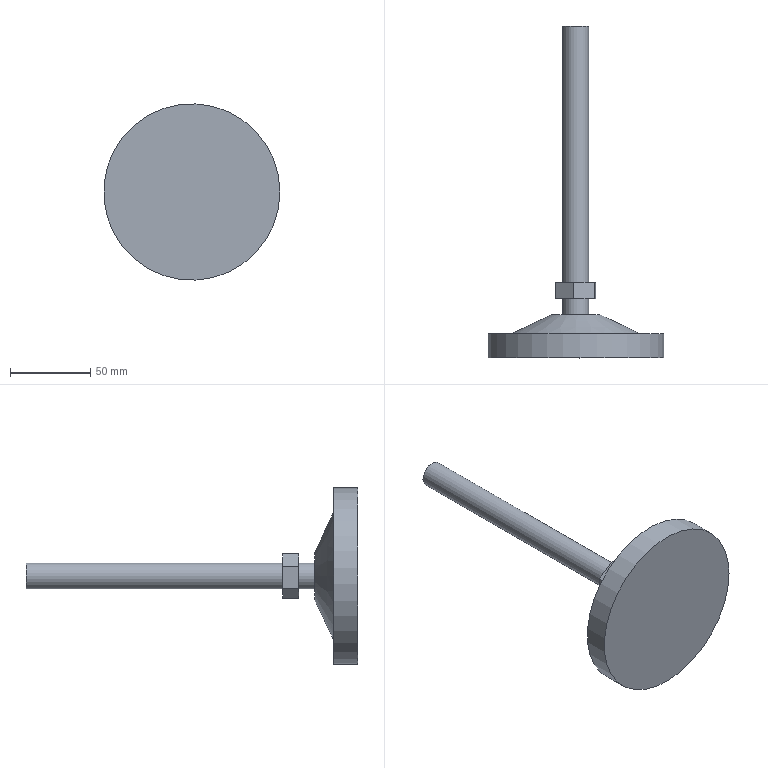Part | STEP file | 17367-articulated foot | 1 solid | 16 faces | box 110 x 207 x 110 mm | volume 212192 mm3 | plane 12 | cylinder 3 | cone 1 | commonest cylinder face diameters 16 x2 110 x1
STEP:
#1=CARTESIAN_POINT('',(0.,0.,0.));
#2=DIRECTION('',(0.,0.,1.));
#3=DIRECTION('',(1.,0.,0.));
#4=AXIS2_PLACEMENT_3D('',#1,#2,#3);
#5=CARTESIAN_POINT('',(1.152,36.982,-13.808));
#6=VERTEX_POINT('',#5);
#7=CARTESIAN_POINT('',(12.535,36.982,-5.906));
#8=VERTEX_POINT('',#7);
#9=CARTESIAN_POINT('',(1.152,36.982,-13.808));
#10=DIRECTION('',(0.8214,0.,0.5703));
#11=VECTOR('',#10,1.);
#12=LINE('',#9,#11);
#13=CARTESIAN_POINT('',(0.,36.982,0.));
#14=DIRECTION('',(0.,1.,0.));
#15=DIRECTION('',(0.,0.,1.));
#16=AXIS2_PLACEMENT_3D('',#13,#14,#15);
#17=PLANE('',#16);
#18=CARTESIAN_POINT('',(-13.808,1.152));
#19=DIRECTION('',(0.5703,0.8214));
#20=VECTOR('',#19,1.);
#21=LINE('',#18,#20);
#22=(GEOMETRIC_REPRESENTATION_CONTEXT(2)PARAMETRIC_REPRESENTATION_CONTEXT()REPRESENTATION_CONTEXT('',''));
#23=DEFINITIONAL_REPRESENTATION('',(#21),#22);
#24=PCURVE('',#17,#23);
#25=CARTESIAN_POINT('',(12.535,36.982,-5.906));
#26=DIRECTION('',(0.5703,0.,-0.8214));
#27=DIRECTION('',(-0.8214,0.,-0.5703));
#28=AXIS2_PLACEMENT_3D('',#25,#26,#27);
#29=PLANE('',#28);
#30=CARTESIAN_POINT('',(13.856,0.));
#31=DIRECTION('',(-1.,0.));
#32=VECTOR('',#31,1.);
#33=LINE('',#30,#32);
#34=(GEOMETRIC_REPRESENTATION_CONTEXT(2)PARAMETRIC_REPRESENTATION_CONTEXT()REPRESENTATION_CONTEXT('',''));
#35=DEFINITIONAL_REPRESENTATION('',(#33),#34);
#36=PCURVE('',#29,#35);
#37=SURFACE_CURVE('',#12,(#24,#36),.PCURVE_S1.);
#38=EDGE_CURVE('',#6,#8,#37,.T.);
#39=ORIENTED_EDGE('',*,*,#38,.F.);
#40=CARTESIAN_POINT('',(-11.382,36.982,-7.902));
#41=VERTEX_POINT('',#40);
#42=CARTESIAN_POINT('',(-11.382,36.982,-7.902));
#43=DIRECTION('',(0.9046,0.,-0.4263));
#44=VECTOR('',#43,1.);
#45=LINE('',#42,#44);
#46=CARTESIAN_POINT('',(-7.902,-11.382));
#47=DIRECTION('',(-0.4263,0.9046));
#48=VECTOR('',#47,1.);
#49=LINE('',#46,#48);
#50=(GEOMETRIC_REPRESENTATION_CONTEXT(2)PARAMETRIC_REPRESENTATION_CONTEXT()REPRESENTATION_CONTEXT('',''));
#51=DEFINITIONAL_REPRESENTATION('',(#49),#50);
#52=PCURVE('',#17,#51);
#53=CARTESIAN_POINT('',(1.152,36.982,-13.808));
#54=DIRECTION('',(-0.4263,0.,-0.9046));
#55=DIRECTION('',(-0.9046,0.,0.4263));
#56=AXIS2_PLACEMENT_3D('',#53,#54,#55);
#57=PLANE('',#56);
#58=CARTESIAN_POINT('',(13.856,0.));
#59=DIRECTION('',(-1.,0.));
#60=VECTOR('',#59,1.);
#61=LINE('',#58,#60);
#62=(GEOMETRIC_REPRESENTATION_CONTEXT(2)PARAMETRIC_REPRESENTATION_CONTEXT()REPRESENTATION_CONTEXT('',''));
#63=DEFINITIONAL_REPRESENTATION('',(#61),#62);
#64=PCURVE('',#57,#63);
#65=SURFACE_CURVE('',#45,(#52,#64),.PCURVE_S1.);
#66=EDGE_CURVE('',#41,#6,#65,.T.);
#67=ORIENTED_EDGE('',*,*,#66,.F.);
#68=CARTESIAN_POINT('',(-12.535,36.982,5.906));
#69=VERTEX_POINT('',#68);
#70=CARTESIAN_POINT('',(-12.535,36.982,5.906));
#71=DIRECTION('',(0.08315,0.,-0.9965));
#72=VECTOR('',#71,1.);
#73=LINE('',#70,#72);
#74=CARTESIAN_POINT('',(5.906,-12.535));
#75=DIRECTION('',(-0.9965,0.08315));
#76=VECTOR('',#75,1.);
#77=LINE('',#74,#76);
#78=(GEOMETRIC_REPRESENTATION_CONTEXT(2)PARAMETRIC_REPRESENTATION_CONTEXT()REPRESENTATION_CONTEXT('',''));
#79=DEFINITIONAL_REPRESENTATION('',(#77),#78);
#80=PCURVE('',#17,#79);
#81=CARTESIAN_POINT('',(-11.382,36.982,-7.902));
#82=DIRECTION('',(-0.9965,0.,-0.08315));
#83=DIRECTION('',(-0.08315,0.,0.9965));
#84=AXIS2_PLACEMENT_3D('',#81,#82,#83);
#85=PLANE('',#84);
#86=CARTESIAN_POINT('',(13.856,0.));
#87=DIRECTION('',(-1.,0.));
#88=VECTOR('',#87,1.);
#89=LINE('',#86,#88);
#90=(GEOMETRIC_REPRESENTATION_CONTEXT(2)PARAMETRIC_REPRESENTATION_CONTEXT()REPRESENTATION_CONTEXT('',''));
#91=DEFINITIONAL_REPRESENTATION('',(#89),#90);
#92=PCURVE('',#85,#91);
#93=SURFACE_CURVE('',#73,(#80,#92),.PCURVE_S1.);
#94=EDGE_CURVE('',#69,#41,#93,.T.);
#95=ORIENTED_EDGE('',*,*,#94,.F.);
#96=CARTESIAN_POINT('',(-1.152,36.982,13.808));
#97=VERTEX_POINT('',#96);
#98=CARTESIAN_POINT('',(-1.152,36.982,13.808));
#99=DIRECTION('',(-0.8214,0.,-0.5703));
#100=VECTOR('',#99,1.);
#101=LINE('',#98,#100);
#102=CARTESIAN_POINT('',(13.808,-1.152));
#103=DIRECTION('',(-0.5703,-0.8214));
#104=VECTOR('',#103,1.);
#105=LINE('',#102,#104);
#106=(GEOMETRIC_REPRESENTATION_CONTEXT(2)PARAMETRIC_REPRESENTATION_CONTEXT()REPRESENTATION_CONTEXT('',''));
#107=DEFINITIONAL_REPRESENTATION('',(#105),#106);
#108=PCURVE('',#17,#107);
#109=CARTESIAN_POINT('',(-12.535,36.982,5.906));
#110=DIRECTION('',(-0.5703,0.,0.8214));
#111=DIRECTION('',(0.8214,0.,0.5703));
#112=AXIS2_PLACEMENT_3D('',#109,#110,#111);
#113=PLANE('',#112);
#114=CARTESIAN_POINT('',(13.856,0.));
#115=DIRECTION('',(-1.,0.));
#116=VECTOR('',#115,1.);
#117=LINE('',#114,#116);
#118=(GEOMETRIC_REPRESENTATION_CONTEXT(2)PARAMETRIC_REPRESENTATION_CONTEXT()REPRESENTATION_CONTEXT('',''));
#119=DEFINITIONAL_REPRESENTATION('',(#117),#118);
#120=PCURVE('',#113,#119);
#121=SURFACE_CURVE('',#101,(#108,#120),.PCURVE_S1.);
#122=EDGE_CURVE('',#97,#69,#121,.T.);
#123=ORIENTED_EDGE('',*,*,#122,.F.);
#124=CARTESIAN_POINT('',(11.382,36.982,7.902));
#125=VERTEX_POINT('',#124);
#126=CARTESIAN_POINT('',(11.382,36.982,7.902));
#127=DIRECTION('',(-0.9046,0.,0.4263));
#128=VECTOR('',#127,1.);
#129=LINE('',#126,#128);
#130=CARTESIAN_POINT('',(7.902,11.382));
#131=DIRECTION('',(0.4263,-0.9046));
#132=VECTOR('',#131,1.);
#133=LINE('',#130,#132);
#134=(GEOMETRIC_REPRESENTATION_CONTEXT(2)PARAMETRIC_REPRESENTATION_CONTEXT()REPRESENTATION_CONTEXT('',''));
#135=DEFINITIONAL_REPRESENTATION('',(#133),#134);
#136=PCURVE('',#17,#135);
#137=CARTESIAN_POINT('',(-1.152,36.982,13.808));
#138=DIRECTION('',(0.4263,0.,0.9046));
#139=DIRECTION('',(0.9046,0.,-0.4263));
#140=AXIS2_PLACEMENT_3D('',#137,#138,#139);
#141=PLANE('',#140);
#142=CARTESIAN_POINT('',(13.856,0.));
#143=DIRECTION('',(-1.,0.));
#144=VECTOR('',#143,1.);
#145=LINE('',#142,#144);
#146=(GEOMETRIC_REPRESENTATION_CONTEXT(2)PARAMETRIC_REPRESENTATION_CONTEXT()REPRESENTATION_CONTEXT('',''));
#147=DEFINITIONAL_REPRESENTATION('',(#145),#146);
#148=PCURVE('',#141,#147);
#149=SURFACE_CURVE('',#129,(#136,#148),.PCURVE_S1.);
#150=EDGE_CURVE('',#125,#97,#149,.T.);
#151=ORIENTED_EDGE('',*,*,#150,.F.);
#152=CARTESIAN_POINT('',(12.535,36.982,-5.906));
#153=DIRECTION('',(-0.08315,0.,0.9965));
#154=VECTOR('',#153,1.);
#155=LINE('',#152,#154);
#156=CARTESIAN_POINT('',(-5.906,12.535));
#157=DIRECTION('',(0.9965,-0.08315));
#158=VECTOR('',#157,1.);
#159=LINE('',#156,#158);
#160=(GEOMETRIC_REPRESENTATION_CONTEXT(2)PARAMETRIC_REPRESENTATION_CONTEXT()REPRESENTATION_CONTEXT('',''));
#161=DEFINITIONAL_REPRESENTATION('',(#159),#160);
#162=PCURVE('',#17,#161);
#163=CARTESIAN_POINT('',(11.382,36.982,7.902));
#164=DIRECTION('',(0.9965,0.,0.08315));
#165=DIRECTION('',(0.08315,0.,-0.9965));
#166=AXIS2_PLACEMENT_3D('',#163,#164,#165);
#167=PLANE('',#166);
#168=CARTESIAN_POINT('',(13.856,0.));
#169=DIRECTION('',(-1.,0.));
#170=VECTOR('',#169,1.);
#171=LINE('',#168,#170);
#172=(GEOMETRIC_REPRESENTATION_CONTEXT(2)PARAMETRIC_REPRESENTATION_CONTEXT()REPRESENTATION_CONTEXT('',''));
#173=DEFINITIONAL_REPRESENTATION('',(#171),#172);
#174=PCURVE('',#167,#173);
#175=SURFACE_CURVE('',#155,(#162,#174),.PCURVE_S1.);
#176=EDGE_CURVE('',#8,#125,#175,.T.);
#177=ORIENTED_EDGE('',*,*,#176,.F.);
#178=EDGE_LOOP('',(#39,#67,#95,#123,#151,#177));
#179=FACE_BOUND('',#178,.T.);
#180=CARTESIAN_POINT('',(-8.,36.982,0.));
#181=VERTEX_POINT('',#180);
#182=CARTESIAN_POINT('',(8.,36.982,0.));
#183=VERTEX_POINT('',#182);
#184=CARTESIAN_POINT('',(0.,36.982,0.));
#185=DIRECTION('',(0.,1.,0.));
#186=DIRECTION('',(1.,0.,0.));
#187=AXIS2_PLACEMENT_3D('',#184,#185,#186);
#188=CIRCLE('',#187,8.);
#189=CARTESIAN_POINT('',(0.,0.));
#190=DIRECTION('',(0.,1.));
#191=AXIS2_PLACEMENT_2D('',#189,#190);
#192=CIRCLE('',#191,8.);
#193=(GEOMETRIC_REPRESENTATION_CONTEXT(2)PARAMETRIC_REPRESENTATION_CONTEXT()REPRESENTATION_CONTEXT('',''));
#194=DEFINITIONAL_REPRESENTATION('',(#192),#193);
#195=PCURVE('',#17,#194);
#196=CARTESIAN_POINT('',(0.,106.982,0.));
#197=DIRECTION('',(0.,-1.,0.));
#198=DIRECTION('',(1.,0.,0.));
#199=AXIS2_PLACEMENT_3D('',#196,#197,#198);
#200=CYLINDRICAL_SURFACE('',#199,8.);
#201=CARTESIAN_POINT('',(6.283,70.));
#202=DIRECTION('',(-1.,0.));
#203=VECTOR('',#202,1.);
#204=LINE('',#201,#203);
#205=(GEOMETRIC_REPRESENTATION_CONTEXT(2)PARAMETRIC_REPRESENTATION_CONTEXT()REPRESENTATION_CONTEXT('',''));
#206=DEFINITIONAL_REPRESENTATION('',(#204),#205);
#207=PCURVE('',#200,#206);
#208=SURFACE_CURVE('',#188,(#195,#207),.PCURVE_S1.);
#209=EDGE_CURVE('',#181,#183,#208,.T.);
#210=ORIENTED_EDGE('',*,*,#209,.F.);
#211=CARTESIAN_POINT('',(0.,36.982,0.));
#212=DIRECTION('',(0.,1.,0.));
#213=DIRECTION('',(1.,0.,0.));
#214=AXIS2_PLACEMENT_3D('',#211,#212,#213);
#215=CIRCLE('',#214,8.);
#216=CARTESIAN_POINT('',(0.,0.));
#217=DIRECTION('',(0.,1.));
#218=AXIS2_PLACEMENT_2D('',#216,#217);
#219=CIRCLE('',#218,8.);
#220=(GEOMETRIC_REPRESENTATION_CONTEXT(2)PARAMETRIC_REPRESENTATION_CONTEXT()REPRESENTATION_CONTEXT('',''));
#221=DEFINITIONAL_REPRESENTATION('',(#219),#220);
#222=PCURVE('',#17,#221);
#223=CARTESIAN_POINT('',(12.566,70.));
#224=DIRECTION('',(-1.,0.));
#225=VECTOR('',#224,1.);
#226=LINE('',#223,#225);
#227=(GEOMETRIC_REPRESENTATION_CONTEXT(2)PARAMETRIC_REPRESENTATION_CONTEXT()REPRESENTATION_CONTEXT('',''));
#228=DEFINITIONAL_REPRESENTATION('',(#226),#227);
#229=PCURVE('',#200,#228);
#230=SURFACE_CURVE('',#215,(#222,#229),.PCURVE_S1.);
#231=EDGE_CURVE('',#183,#181,#230,.T.);
#232=ORIENTED_EDGE('',*,*,#231,.F.);
#233=EDGE_LOOP('',(#210,#232));
#234=FACE_BOUND('',#233,.T.);
#235=ADVANCED_FACE('',(#179,#234),#17,.T.);
#236=CARTESIAN_POINT('',(1.152,26.982,-13.808));
#237=VERTEX_POINT('',#236);
#238=CARTESIAN_POINT('',(-11.382,26.982,-7.902));
#239=VERTEX_POINT('',#238);
#240=CARTESIAN_POINT('',(1.152,26.982,-13.808));
#241=DIRECTION('',(-0.9046,0.,0.4263));
#242=VECTOR('',#241,1.);
#243=LINE('',#240,#242);
#244=CARTESIAN_POINT('',(0.,26.982,0.));
#245=DIRECTION('',(0.,1.,0.));
#246=DIRECTION('',(0.,0.,1.));
#247=AXIS2_PLACEMENT_3D('',#244,#245,#246);
#248=PLANE('',#247);
#249=CARTESIAN_POINT('',(-13.808,1.152));
#250=DIRECTION('',(0.4263,-0.9046));
#251=VECTOR('',#250,1.);
#252=LINE('',#249,#251);
#253=(GEOMETRIC_REPRESENTATION_CONTEXT(2)PARAMETRIC_REPRESENTATION_CONTEXT()REPRESENTATION_CONTEXT('',''));
#254=DEFINITIONAL_REPRESENTATION('',(#252),#253);
#255=PCURVE('',#248,#254);
#256=CARTESIAN_POINT('',(0.,-10.));
#257=DIRECTION('',(1.,0.));
#258=VECTOR('',#257,1.);
#259=LINE('',#256,#258);
#260=(GEOMETRIC_REPRESENTATION_CONTEXT(2)PARAMETRIC_REPRESENTATION_CONTEXT()REPRESENTATION_CONTEXT('',''));
#261=DEFINITIONAL_REPRESENTATION('',(#259),#260);
#262=PCURVE('',#57,#261);
#263=SURFACE_CURVE('',#243,(#255,#262),.PCURVE_S1.);
#264=EDGE_CURVE('',#237,#239,#263,.T.);
#265=ORIENTED_EDGE('',*,*,#264,.F.);
#266=CARTESIAN_POINT('',(12.535,26.982,-5.906));
#267=VERTEX_POINT('',#266);
#268=CARTESIAN_POINT('',(12.535,26.982,-5.906));
#269=DIRECTION('',(-0.8214,0.,-0.5703));
#270=VECTOR('',#269,1.);
#271=LINE('',#268,#270);
#272=CARTESIAN_POINT('',(-5.906,12.535));
#273=DIRECTION('',(-0.5703,-0.8214));
#274=VECTOR('',#273,1.);
#275=LINE('',#272,#274);
#276=(GEOMETRIC_REPRESENTATION_CONTEXT(2)PARAMETRIC_REPRESENTATION_CONTEXT()REPRESENTATION_CONTEXT('',''));
#277=DEFINITIONAL_REPRESENTATION('',(#275),#276);
#278=PCURVE('',#248,#277);
#279=CARTESIAN_POINT('',(0.,-10.));
#280=DIRECTION('',(1.,0.));
#281=VECTOR('',#280,1.);
#282=LINE('',#279,#281);
#283=(GEOMETRIC_REPRESENTATION_CONTEXT(2)PARAMETRIC_REPRESENTATION_CONTEXT()REPRESENTATION_CONTEXT('',''));
#284=DEFINITIONAL_REPRESENTATION('',(#282),#283);
#285=PCURVE('',#29,#284);
#286=SURFACE_CURVE('',#271,(#278,#285),.PCURVE_S1.);
#287=EDGE_CURVE('',#267,#237,#286,.T.);
#288=ORIENTED_EDGE('',*,*,#287,.F.);
#289=CARTESIAN_POINT('',(11.382,26.982,7.902));
#290=VERTEX_POINT('',#289);
#291=CARTESIAN_POINT('',(11.382,26.982,7.902));
#292=DIRECTION('',(0.08315,0.,-0.9965));
#293=VECTOR('',#292,1.);
#294=LINE('',#291,#293);
#295=CARTESIAN_POINT('',(7.902,11.382));
#296=DIRECTION('',(-0.9965,0.08315));
#297=VECTOR('',#296,1.);
#298=LINE('',#295,#297);
#299=(GEOMETRIC_REPRESENTATION_CONTEXT(2)PARAMETRIC_REPRESENTATION_CONTEXT()REPRESENTATION_CONTEXT('',''));
#300=DEFINITIONAL_REPRESENTATION('',(#298),#299);
#301=PCURVE('',#248,#300);
#302=CARTESIAN_POINT('',(0.,-10.));
#303=DIRECTION('',(1.,0.));
#304=VECTOR('',#303,1.);
#305=LINE('',#302,#304);
#306=(GEOMETRIC_REPRESENTATION_CONTEXT(2)PARAMETRIC_REPRESENTATION_CONTEXT()REPRESENTATION_CONTEXT('',''));
#307=DEFINITIONAL_REPRESENTATION('',(#305),#306);
#308=PCURVE('',#167,#307);
#309=SURFACE_CURVE('',#294,(#301,#308),.PCURVE_S1.);
#310=EDGE_CURVE('',#290,#267,#309,.T.);
#311=ORIENTED_EDGE('',*,*,#310,.F.);
#312=CARTESIAN_POINT('',(-1.152,26.982,13.808));
#313=VERTEX_POINT('',#312);
#314=CARTESIAN_POINT('',(-1.152,26.982,13.808));
#315=DIRECTION('',(0.9046,0.,-0.4263));
#316=VECTOR('',#315,1.);
#317=LINE('',#314,#316);
#318=CARTESIAN_POINT('',(13.808,-1.152));
#319=DIRECTION('',(-0.4263,0.9046));
#320=VECTOR('',#319,1.);
#321=LINE('',#318,#320);
#322=(GEOMETRIC_REPRESENTATION_CONTEXT(2)PARAMETRIC_REPRESENTATION_CONTEXT()REPRESENTATION_CONTEXT('',''));
#323=DEFINITIONAL_REPRESENTATION('',(#321),#322);
#324=PCURVE('',#248,#323);
#325=CARTESIAN_POINT('',(0.,-10.));
#326=DIRECTION('',(1.,0.));
#327=VECTOR('',#326,1.);
#328=LINE('',#325,#327);
#329=(GEOMETRIC_REPRESENTATION_CONTEXT(2)PARAMETRIC_REPRESENTATION_CONTEXT()REPRESENTATION_CONTEXT('',''));
#330=DEFINITIONAL_REPRESENTATION('',(#328),#329);
#331=PCURVE('',#141,#330);
#332=SURFACE_CURVE('',#317,(#324,#331),.PCURVE_S1.);
#333=EDGE_CURVE('',#313,#290,#332,.T.);
#334=ORIENTED_EDGE('',*,*,#333,.F.);
#335=CARTESIAN_POINT('',(-12.535,26.982,5.906));
#336=VERTEX_POINT('',#335);
#337=CARTESIAN_POINT('',(-12.535,26.982,5.906));
#338=DIRECTION('',(0.8214,0.,0.5703));
#339=VECTOR('',#338,1.);
#340=LINE('',#337,#339);
#341=CARTESIAN_POINT('',(5.906,-12.535));
#342=DIRECTION('',(0.5703,0.8214));
#343=VECTOR('',#342,1.);
#344=LINE('',#341,#343);
#345=(GEOMETRIC_REPRESENTATION_CONTEXT(2)PARAMETRIC_REPRESENTATION_CONTEXT()REPRESENTATION_CONTEXT('',''));
#346=DEFINITIONAL_REPRESENTATION('',(#344),#345);
#347=PCURVE('',#248,#346);
#348=CARTESIAN_POINT('',(0.,-10.));
#349=DIRECTION('',(1.,0.));
#350=VECTOR('',#349,1.);
#351=LINE('',#348,#350);
#352=(GEOMETRIC_REPRESENTATION_CONTEXT(2)PARAMETRIC_REPRESENTATION_CONTEXT()REPRESENTATION_CONTEXT('',''));
#353=DEFINITIONAL_REPRESENTATION('',(#351),#352);
#354=PCURVE('',#113,#353);
#355=SURFACE_CURVE('',#340,(#347,#354),.PCURVE_S1.);
#356=EDGE_CURVE('',#336,#313,#355,.T.);
#357=ORIENTED_EDGE('',*,*,#356,.F.);
#358=CARTESIAN_POINT('',(-11.382,26.982,-7.902));
#359=DIRECTION('',(-0.08315,0.,0.9965));
#360=VECTOR('',#359,1.);
#361=LINE('',#358,#360);
#362=CARTESIAN_POINT('',(-7.902,-11.382));
#363=DIRECTION('',(0.9965,-0.08315));
#364=VECTOR('',#363,1.);
#365=LINE('',#362,#364);
#366=(GEOMETRIC_REPRESENTATION_CONTEXT(2)PARAMETRIC_REPRESENTATION_CONTEXT()REPRESENTATION_CONTEXT('',''));
#367=DEFINITIONAL_REPRESENTATION('',(#365),#366);
#368=PCURVE('',#248,#367);
#369=CARTESIAN_POINT('',(0.,-10.));
#370=DIRECTION('',(1.,0.));
#371=VECTOR('',#370,1.);
#372=LINE('',#369,#371);
#373=(GEOMETRIC_REPRESENTATION_CONTEXT(2)PARAMETRIC_REPRESENTATION_CONTEXT()REPRESENTATION_CONTEXT('',''));
#374=DEFINITIONAL_REPRESENTATION('',(#372),#373);
#375=PCURVE('',#85,#374);
#376=SURFACE_CURVE('',#361,(#368,#375),.PCURVE_S1.);
#377=EDGE_CURVE('',#239,#336,#376,.T.);
#378=ORIENTED_EDGE('',*,*,#377,.F.);
#379=EDGE_LOOP('',(#265,#288,#311,#334,#357,#378));
#380=FACE_BOUND('',#379,.T.);
#381=CARTESIAN_POINT('',(-8.,26.982,0.));
#382=VERTEX_POINT('',#381);
#383=CARTESIAN_POINT('',(8.,26.982,0.));
#384=VERTEX_POINT('',#383);
#385=CARTESIAN_POINT('',(0.,26.982,0.));
#386=DIRECTION('',(0.,-1.,0.));
#387=DIRECTION('',(1.,0.,0.));
#388=AXIS2_PLACEMENT_3D('',#385,#386,#387);
#389=CIRCLE('',#388,8.);
#390=CARTESIAN_POINT('',(0.,8.));
#391=CARTESIAN_POINT('',(13.856,8.));
#392=CARTESIAN_POINT('',(6.928,-4.));
#393=CARTESIAN_POINT('',(0.,-16.));
#394=CARTESIAN_POINT('',(-6.928,-4.));
#395=CARTESIAN_POINT('',(-13.856,8.));
#396=CARTESIAN_POINT('',(0.,8.));
#397=(BOUNDED_CURVE()B_SPLINE_CURVE(2,(#390,#391,#392,#393,#394,#395,#396),.UNSPECIFIED.,.T.,.F.)B_SPLINE_CURVE_WITH_KNOTS((1,2,2,2,2,1),(-2.094,0.,2.094,4.189,6.283,8.378),.UNSPECIFIED.)CURVE()GEOMETRIC_REPRESENTATION_ITEM()RATIONAL_B_SPLINE_CURVE((1.,0.5,1.,0.5,1.,0.5,1.))REPRESENTATION_ITEM(''));
#398=(GEOMETRIC_REPRESENTATION_CONTEXT(2)PARAMETRIC_REPRESENTATION_CONTEXT()REPRESENTATION_CONTEXT('',''));
#399=DEFINITIONAL_REPRESENTATION('',(#397),#398);
#400=PCURVE('',#248,#399);
#401=CARTESIAN_POINT('',(0.,106.982,0.));
#402=DIRECTION('',(0.,-1.,0.));
#403=DIRECTION('',(1.,0.,0.));
#404=AXIS2_PLACEMENT_3D('',#401,#402,#403);
#405=CYLINDRICAL_SURFACE('',#404,8.);
#406=CARTESIAN_POINT('',(0.,80.));
#407=DIRECTION('',(1.,0.));
#408=VECTOR('',#407,1.);
#409=LINE('',#406,#408);
#410=(GEOMETRIC_REPRESENTATION_CONTEXT(2)PARAMETRIC_REPRESENTATION_CONTEXT()REPRESENTATION_CONTEXT('',''));
#411=DEFINITIONAL_REPRESENTATION('',(#409),#410);
#412=PCURVE('',#405,#411);
#413=SURFACE_CURVE('',#389,(#400,#412),.PCURVE_S1.);
#414=EDGE_CURVE('',#382,#384,#413,.T.);
#415=ORIENTED_EDGE('',*,*,#414,.F.);
#416=CARTESIAN_POINT('',(0.,26.982,0.));
#417=DIRECTION('',(0.,-1.,0.));
#418=DIRECTION('',(1.,0.,0.));
#419=AXIS2_PLACEMENT_3D('',#416,#417,#418);
#420=CIRCLE('',#419,8.);
#421=CARTESIAN_POINT('',(0.,8.));
#422=CARTESIAN_POINT('',(13.856,8.));
#423=CARTESIAN_POINT('',(6.928,-4.));
#424=CARTESIAN_POINT('',(0.,-16.));
#425=CARTESIAN_POINT('',(-6.928,-4.));
#426=CARTESIAN_POINT('',(-13.856,8.));
#427=CARTESIAN_POINT('',(0.,8.));
#428=(BOUNDED_CURVE()B_SPLINE_CURVE(2,(#421,#422,#423,#424,#425,#426,#427),.UNSPECIFIED.,.T.,.F.)B_SPLINE_CURVE_WITH_KNOTS((1,2,2,2,2,1),(-2.094,0.,2.094,4.189,6.283,8.378),.UNSPECIFIED.)CURVE()GEOMETRIC_REPRESENTATION_ITEM()RATIONAL_B_SPLINE_CURVE((1.,0.5,1.,0.5,1.,0.5,1.))REPRESENTATION_ITEM(''));
#429=(GEOMETRIC_REPRESENTATION_CONTEXT(2)PARAMETRIC_REPRESENTATION_CONTEXT()REPRESENTATION_CONTEXT('',''));
#430=DEFINITIONAL_REPRESENTATION('',(#428),#429);
#431=PCURVE('',#248,#430);
#432=CARTESIAN_POINT('',(-6.283,80.));
#433=DIRECTION('',(1.,0.));
#434=VECTOR('',#433,1.);
#435=LINE('',#432,#434);
#436=(GEOMETRIC_REPRESENTATION_CONTEXT(2)PARAMETRIC_REPRESENTATION_CONTEXT()REPRESENTATION_CONTEXT('',''));
#437=DEFINITIONAL_REPRESENTATION('',(#435),#436);
#438=PCURVE('',#405,#437);
#439=SURFACE_CURVE('',#420,(#431,#438),.PCURVE_S1.);
#440=EDGE_CURVE('',#384,#382,#439,.T.);
#441=ORIENTED_EDGE('',*,*,#440,.F.);
#442=EDGE_LOOP('',(#415,#441));
#443=FACE_BOUND('',#442,.T.);
#444=ADVANCED_FACE('',(#380,#443),#248,.F.);
#445=ORIENTED_EDGE('',*,*,#264,.T.);
#446=CARTESIAN_POINT('',(-11.382,36.982,-7.902));
#447=DIRECTION('',(0.,-1.,0.));
#448=VECTOR('',#447,1.);
#449=LINE('',#446,#448);
#450=CARTESIAN_POINT('',(13.856,0.));
#451=DIRECTION('',(0.,-1.));
#452=VECTOR('',#451,1.);
#453=LINE('',#450,#452);
#454=(GEOMETRIC_REPRESENTATION_CONTEXT(2)PARAMETRIC_REPRESENTATION_CONTEXT()REPRESENTATION_CONTEXT('',''));
#455=DEFINITIONAL_REPRESENTATION('',(#453),#454);
#456=PCURVE('',#57,#455);
#457=CARTESIAN_POINT('',(0.,0.));
#458=DIRECTION('',(0.,-1.));
#459=VECTOR('',#458,1.);
#460=LINE('',#457,#459);
#461=(GEOMETRIC_REPRESENTATION_CONTEXT(2)PARAMETRIC_REPRESENTATION_CONTEXT()REPRESENTATION_CONTEXT('',''));
#462=DEFINITIONAL_REPRESENTATION('',(#460),#461);
#463=PCURVE('',#85,#462);
#464=SURFACE_CURVE('',#449,(#456,#463),.PCURVE_S1.);
#465=EDGE_CURVE('',#41,#239,#464,.T.);
#466=ORIENTED_EDGE('',*,*,#465,.F.);
#467=ORIENTED_EDGE('',*,*,#66,.T.);
#468=CARTESIAN_POINT('',(1.152,36.982,-13.808));
#469=DIRECTION('',(0.,-1.,0.));
#470=VECTOR('',#469,1.);
#471=LINE('',#468,#470);
#472=CARTESIAN_POINT('',(0.,0.));
#473=DIRECTION('',(0.,-1.));
#474=VECTOR('',#473,1.);
#475=LINE('',#472,#474);
#476=(GEOMETRIC_REPRESENTATION_CONTEXT(2)PARAMETRIC_REPRESENTATION_CONTEXT()REPRESENTATION_CONTEXT('',''));
#477=DEFINITIONAL_REPRESENTATION('',(#475),#476);
#478=PCURVE('',#57,#477);
#479=CARTESIAN_POINT('',(13.856,0.));
#480=DIRECTION('',(0.,-1.));
#481=VECTOR('',#480,1.);
#482=LINE('',#479,#481);
#483=(GEOMETRIC_REPRESENTATION_CONTEXT(2)PARAMETRIC_REPRESENTATION_CONTEXT()REPRESENTATION_CONTEXT('',''));
#484=DEFINITIONAL_REPRESENTATION('',(#482),#483);
#485=PCURVE('',#29,#484);
#486=SURFACE_CURVE('',#471,(#478,#485),.PCURVE_S1.);
#487=EDGE_CURVE('',#6,#237,#486,.T.);
#488=ORIENTED_EDGE('',*,*,#487,.T.);
#489=EDGE_LOOP('',(#445,#466,#467,#488));
#490=FACE_BOUND('',#489,.T.);
#491=ADVANCED_FACE('',(#490),#57,.T.);
#492=ORIENTED_EDGE('',*,*,#377,.T.);
#493=CARTESIAN_POINT('',(-12.535,36.982,5.906));
#494=DIRECTION('',(0.,-1.,0.));
#495=VECTOR('',#494,1.);
#496=LINE('',#493,#495);
#497=CARTESIAN_POINT('',(13.856,0.));
#498=DIRECTION('',(0.,-1.));
#499=VECTOR('',#498,1.);
#500=LINE('',#497,#499);
#501=(GEOMETRIC_REPRESENTATION_CONTEXT(2)PARAMETRIC_REPRESENTATION_CONTEXT()REPRESENTATION_CONTEXT('',''));
#502=DEFINITIONAL_REPRESENTATION('',(#500),#501);
#503=PCURVE('',#85,#502);
#504=CARTESIAN_POINT('',(0.,0.));
#505=DIRECTION('',(0.,-1.));
#506=VECTOR('',#505,1.);
#507=LINE('',#504,#506);
#508=(GEOMETRIC_REPRESENTATION_CONTEXT(2)PARAMETRIC_REPRESENTATION_CONTEXT()REPRESENTATION_CONTEXT('',''));
#509=DEFINITIONAL_REPRESENTATION('',(#507),#508);
#510=PCURVE('',#113,#509);
#511=SURFACE_CURVE('',#496,(#503,#510),.PCURVE_S1.);
#512=EDGE_CURVE('',#69,#336,#511,.T.);
#513=ORIENTED_EDGE('',*,*,#512,.F.);
#514=ORIENTED_EDGE('',*,*,#94,.T.);
#515=ORIENTED_EDGE('',*,*,#465,.T.);
#516=EDGE_LOOP('',(#492,#513,#514,#515));
#517=FACE_BOUND('',#516,.T.);
#518=ADVANCED_FACE('',(#517),#85,.T.);
#519=ORIENTED_EDGE('',*,*,#356,.T.);
#520=CARTESIAN_POINT('',(-1.152,36.982,13.808));
#521=DIRECTION('',(0.,-1.,0.));
#522=VECTOR('',#521,1.);
#523=LINE('',#520,#522);
#524=CARTESIAN_POINT('',(13.856,0.));
#525=DIRECTION('',(0.,-1.));
#526=VECTOR('',#525,1.);
#527=LINE('',#524,#526);
#528=(GEOMETRIC_REPRESENTATION_CONTEXT(2)PARAMETRIC_REPRESENTATION_CONTEXT()REPRESENTATION_CONTEXT('',''));
#529=DEFINITIONAL_REPRESENTATION('',(#527),#528);
#530=PCURVE('',#113,#529);
#531=CARTESIAN_POINT('',(0.,0.));
#532=DIRECTION('',(0.,-1.));
#533=VECTOR('',#532,1.);
#534=LINE('',#531,#533);
#535=(GEOMETRIC_REPRESENTATION_CONTEXT(2)PARAMETRIC_REPRESENTATION_CONTEXT()REPRESENTATION_CONTEXT('',''));
#536=DEFINITIONAL_REPRESENTATION('',(#534),#535);
#537=PCURVE('',#141,#536);
#538=SURFACE_CURVE('',#523,(#530,#537),.PCURVE_S1.);
#539=EDGE_CURVE('',#97,#313,#538,.T.);
#540=ORIENTED_EDGE('',*,*,#539,.F.);
#541=ORIENTED_EDGE('',*,*,#122,.T.);
#542=ORIENTED_EDGE('',*,*,#512,.T.);
#543=EDGE_LOOP('',(#519,#540,#541,#542));
#544=FACE_BOUND('',#543,.T.);
#545=ADVANCED_FACE('',(#544),#113,.T.);
#546=ORIENTED_EDGE('',*,*,#333,.T.);
#547=CARTESIAN_POINT('',(11.382,36.982,7.902));
#548=DIRECTION('',(0.,-1.,0.));
#549=VECTOR('',#548,1.);
#550=LINE('',#547,#549);
#551=CARTESIAN_POINT('',(13.856,0.));
#552=DIRECTION('',(0.,-1.));
#553=VECTOR('',#552,1.);
#554=LINE('',#551,#553);
#555=(GEOMETRIC_REPRESENTATION_CONTEXT(2)PARAMETRIC_REPRESENTATION_CONTEXT()REPRESENTATION_CONTEXT('',''));
#556=DEFINITIONAL_REPRESENTATION('',(#554),#555);
#557=PCURVE('',#141,#556);
#558=CARTESIAN_POINT('',(0.,0.));
#559=DIRECTION('',(0.,-1.));
#560=VECTOR('',#559,1.);
#561=LINE('',#558,#560);
#562=(GEOMETRIC_REPRESENTATION_CONTEXT(2)PARAMETRIC_REPRESENTATION_CONTEXT()REPRESENTATION_CONTEXT('',''));
#563=DEFINITIONAL_REPRESENTATION('',(#561),#562);
#564=PCURVE('',#167,#563);
#565=SURFACE_CURVE('',#550,(#557,#564),.PCURVE_S1.);
#566=EDGE_CURVE('',#125,#290,#565,.T.);
#567=ORIENTED_EDGE('',*,*,#566,.F.);
#568=ORIENTED_EDGE('',*,*,#150,.T.);
#569=ORIENTED_EDGE('',*,*,#539,.T.);
#570=EDGE_LOOP('',(#546,#567,#568,#569));
#571=FACE_BOUND('',#570,.T.);
#572=ADVANCED_FACE('',(#571),#141,.T.);
#573=ORIENTED_EDGE('',*,*,#310,.T.);
#574=CARTESIAN_POINT('',(12.535,36.982,-5.906));
#575=DIRECTION('',(0.,-1.,0.));
#576=VECTOR('',#575,1.);
#577=LINE('',#574,#576);
#578=CARTESIAN_POINT('',(13.856,0.));
#579=DIRECTION('',(0.,-1.));
#580=VECTOR('',#579,1.);
#581=LINE('',#578,#580);
#582=(GEOMETRIC_REPRESENTATION_CONTEXT(2)PARAMETRIC_REPRESENTATION_CONTEXT()REPRESENTATION_CONTEXT('',''));
#583=DEFINITIONAL_REPRESENTATION('',(#581),#582);
#584=PCURVE('',#167,#583);
#585=CARTESIAN_POINT('',(0.,0.));
#586=DIRECTION('',(0.,-1.));
#587=VECTOR('',#586,1.);
#588=LINE('',#585,#587);
#589=(GEOMETRIC_REPRESENTATION_CONTEXT(2)PARAMETRIC_REPRESENTATION_CONTEXT()REPRESENTATION_CONTEXT('',''));
#590=DEFINITIONAL_REPRESENTATION('',(#588),#589);
#591=PCURVE('',#29,#590);
#592=SURFACE_CURVE('',#577,(#584,#591),.PCURVE_S1.);
#593=EDGE_CURVE('',#8,#267,#592,.T.);
#594=ORIENTED_EDGE('',*,*,#593,.F.);
#595=ORIENTED_EDGE('',*,*,#176,.T.);
#596=ORIENTED_EDGE('',*,*,#566,.T.);
#597=EDGE_LOOP('',(#573,#594,#595,#596));
#598=FACE_BOUND('',#597,.T.);
#599=ADVANCED_FACE('',(#598),#167,.T.);
#600=ORIENTED_EDGE('',*,*,#287,.T.);
#601=ORIENTED_EDGE('',*,*,#487,.F.);
#602=ORIENTED_EDGE('',*,*,#38,.T.);
#603=ORIENTED_EDGE('',*,*,#593,.T.);
#604=EDGE_LOOP('',(#600,#601,#602,#603));
#605=FACE_BOUND('',#604,.T.);
#606=ADVANCED_FACE('',(#605),#29,.T.);
#607=CARTESIAN_POINT('',(8.,16.982,0.));
#608=VERTEX_POINT('',#607);
#609=CARTESIAN_POINT('',(0.,16.982,0.));
#610=DIRECTION('',(0.,-1.,0.));
#611=DIRECTION('',(1.,0.,0.));
#612=AXIS2_PLACEMENT_3D('',#609,#610,#611);
#613=CIRCLE('',#612,8.);
#614=CARTESIAN_POINT('',(0.,90.));
#615=DIRECTION('',(1.,0.));
#616=VECTOR('',#615,1.);
#617=LINE('',#614,#616);
#618=(GEOMETRIC_REPRESENTATION_CONTEXT(2)PARAMETRIC_REPRESENTATION_CONTEXT()REPRESENTATION_CONTEXT('',''));
#619=DEFINITIONAL_REPRESENTATION('',(#617),#618);
#620=PCURVE('',#405,#619);
#621=CARTESIAN_POINT('',(11.5,16.982,0.));
#622=DIRECTION('',(0.,1.,0.));
#623=DIRECTION('',(0.,0.,1.));
#624=AXIS2_PLACEMENT_3D('',#621,#622,#623);
#625=PLANE('',#624);
#626=CARTESIAN_POINT('',(0.,-3.5));
#627=CARTESIAN_POINT('',(13.856,-3.5));
#628=CARTESIAN_POINT('',(6.928,-15.5));
#629=CARTESIAN_POINT('',(0.,-27.5));
#630=CARTESIAN_POINT('',(-6.928,-15.5));
#631=CARTESIAN_POINT('',(-13.856,-3.5));
#632=CARTESIAN_POINT('',(0.,-3.5));
#633=(BOUNDED_CURVE()B_SPLINE_CURVE(2,(#626,#627,#628,#629,#630,#631,#632),.UNSPECIFIED.,.T.,.F.)B_SPLINE_CURVE_WITH_KNOTS((1,2,2,2,2,1),(-2.094,0.,2.094,4.189,6.283,8.378),.UNSPECIFIED.)CURVE()GEOMETRIC_REPRESENTATION_ITEM()RATIONAL_B_SPLINE_CURVE((1.,0.5,1.,0.5,1.,0.5,1.))REPRESENTATION_ITEM(''));
#634=(GEOMETRIC_REPRESENTATION_CONTEXT(2)PARAMETRIC_REPRESENTATION_CONTEXT()REPRESENTATION_CONTEXT('',''));
#635=DEFINITIONAL_REPRESENTATION('',(#633),#634);
#636=PCURVE('',#625,#635);
#637=SURFACE_CURVE('',#613,(#620,#636),.PCURVE_S1.);
#638=EDGE_CURVE('',#608,#608,#637,.T.);
#639=ORIENTED_EDGE('',*,*,#638,.F.);
#640=CARTESIAN_POINT('',(8.,26.982,0.));
#641=CARTESIAN_POINT('',(8.,16.982,0.));
#642=B_SPLINE_CURVE_WITH_KNOTS('',1,(#640,#641),.UNSPECIFIED.,.F.,.F.,(2,2),(80.,90.),.PIECEWISE_BEZIER_KNOTS.);
#643=CARTESIAN_POINT('',(0.,0.));
#644=DIRECTION('',(0.,1.));
#645=VECTOR('',#644,1.);
#646=LINE('',#643,#645);
#647=(GEOMETRIC_REPRESENTATION_CONTEXT(2)PARAMETRIC_REPRESENTATION_CONTEXT()REPRESENTATION_CONTEXT('',''));
#648=DEFINITIONAL_REPRESENTATION('',(#646),#647);
#649=PCURVE('',#405,#648);
#650=CARTESIAN_POINT('',(6.283,0.));
#651=DIRECTION('',(0.,1.));
#652=VECTOR('',#651,1.);
#653=LINE('',#650,#652);
#654=(GEOMETRIC_REPRESENTATION_CONTEXT(2)PARAMETRIC_REPRESENTATION_CONTEXT()REPRESENTATION_CONTEXT('',''));
#655=DEFINITIONAL_REPRESENTATION('',(#653),#654);
#656=PCURVE('',#405,#655);
#657=SEAM_CURVE('',#642,(#649,#656),.PCURVE_S1.);
#658=EDGE_CURVE('',#384,#608,#657,.T.);
#659=ORIENTED_EDGE('',*,*,#658,.F.);
#660=ORIENTED_EDGE('',*,*,#440,.T.);
#661=ORIENTED_EDGE('',*,*,#414,.T.);
#662=ORIENTED_EDGE('',*,*,#658,.T.);
#663=EDGE_LOOP('',(#639,#659,#660,#661,#662));
#664=FACE_BOUND('',#663,.T.);
#665=ADVANCED_FACE('',(#664),#405,.T.);
#666=CARTESIAN_POINT('',(8.,196.982,0.));
#667=VERTEX_POINT('',#666);
#668=CARTESIAN_POINT('',(0.,196.982,0.));
#669=DIRECTION('',(0.,-1.,0.));
#670=DIRECTION('',(1.,0.,0.));
#671=AXIS2_PLACEMENT_3D('',#668,#669,#670);
#672=CIRCLE('',#671,8.);
#673=CARTESIAN_POINT('',(4.,196.982,0.));
#674=DIRECTION('',(0.,1.,0.));
#675=DIRECTION('',(0.,0.,1.));
#676=AXIS2_PLACEMENT_3D('',#673,#674,#675);
#677=PLANE('',#676);
#678=CARTESIAN_POINT('',(0.,4.));
#679=CARTESIAN_POINT('',(13.856,4.));
#680=CARTESIAN_POINT('',(6.928,-8.));
#681=CARTESIAN_POINT('',(0.,-20.));
#682=CARTESIAN_POINT('',(-6.928,-8.));
#683=CARTESIAN_POINT('',(-13.856,4.));
#684=CARTESIAN_POINT('',(0.,4.));
#685=(BOUNDED_CURVE()B_SPLINE_CURVE(2,(#678,#679,#680,#681,#682,#683,#684),.UNSPECIFIED.,.T.,.F.)B_SPLINE_CURVE_WITH_KNOTS((1,2,2,2,2,1),(-2.094,0.,2.094,4.189,6.283,8.378),.UNSPECIFIED.)CURVE()GEOMETRIC_REPRESENTATION_ITEM()RATIONAL_B_SPLINE_CURVE((1.,0.5,1.,0.5,1.,0.5,1.))REPRESENTATION_ITEM(''));
#686=(GEOMETRIC_REPRESENTATION_CONTEXT(2)PARAMETRIC_REPRESENTATION_CONTEXT()REPRESENTATION_CONTEXT('',''));
#687=DEFINITIONAL_REPRESENTATION('',(#685),#686);
#688=PCURVE('',#677,#687);
#689=CARTESIAN_POINT('',(0.,-90.));
#690=DIRECTION('',(1.,0.));
#691=VECTOR('',#690,1.);
#692=LINE('',#689,#691);
#693=(GEOMETRIC_REPRESENTATION_CONTEXT(2)PARAMETRIC_REPRESENTATION_CONTEXT()REPRESENTATION_CONTEXT('',''));
#694=DEFINITIONAL_REPRESENTATION('',(#692),#693);
#695=PCURVE('',#200,#694);
#696=SURFACE_CURVE('',#672,(#688,#695),.PCURVE_S1.);
#697=EDGE_CURVE('',#667,#667,#696,.T.);
#698=ORIENTED_EDGE('',*,*,#697,.F.);
#699=EDGE_LOOP('',(#698));
#700=FACE_BOUND('',#699,.T.);
#701=ADVANCED_FACE('',(#700),#677,.T.);
#702=ORIENTED_EDGE('',*,*,#209,.T.);
#703=CARTESIAN_POINT('',(8.,196.982,0.));
#704=CARTESIAN_POINT('',(8.,36.982,0.));
#705=B_SPLINE_CURVE_WITH_KNOTS('',1,(#703,#704),.UNSPECIFIED.,.F.,.F.,(2,2),(-90.,70.),.PIECEWISE_BEZIER_KNOTS.);
#706=CARTESIAN_POINT('',(0.,0.));
#707=DIRECTION('',(0.,1.));
#708=VECTOR('',#707,1.);
#709=LINE('',#706,#708);
#710=(GEOMETRIC_REPRESENTATION_CONTEXT(2)PARAMETRIC_REPRESENTATION_CONTEXT()REPRESENTATION_CONTEXT('',''));
#711=DEFINITIONAL_REPRESENTATION('',(#709),#710);
#712=PCURVE('',#200,#711);
#713=CARTESIAN_POINT('',(6.283,0.));
#714=DIRECTION('',(0.,1.));
#715=VECTOR('',#714,1.);
#716=LINE('',#713,#715);
#717=(GEOMETRIC_REPRESENTATION_CONTEXT(2)PARAMETRIC_REPRESENTATION_CONTEXT()REPRESENTATION_CONTEXT('',''));
#718=DEFINITIONAL_REPRESENTATION('',(#716),#717);
#719=PCURVE('',#200,#718);
#720=SEAM_CURVE('',#705,(#712,#719),.PCURVE_S1.);
#721=EDGE_CURVE('',#667,#183,#720,.T.);
#722=ORIENTED_EDGE('',*,*,#721,.F.);
#723=ORIENTED_EDGE('',*,*,#697,.T.);
#724=ORIENTED_EDGE('',*,*,#721,.T.);
#725=ORIENTED_EDGE('',*,*,#231,.T.);
#726=EDGE_LOOP('',(#702,#722,#723,#724,#725));
#727=FACE_BOUND('',#726,.T.);
#728=ADVANCED_FACE('',(#727),#200,.T.);
#729=CARTESIAN_POINT('',(15.,16.982,0.));
#730=VERTEX_POINT('',#729);
#731=CARTESIAN_POINT('',(0.,16.982,0.));
#732=DIRECTION('',(0.,-1.,0.));
#733=DIRECTION('',(1.,0.,0.));
#734=AXIS2_PLACEMENT_3D('',#731,#732,#733);
#735=CIRCLE('',#734,15.);
#736=CARTESIAN_POINT('',(0.,3.5));
#737=CARTESIAN_POINT('',(25.981,3.5));
#738=CARTESIAN_POINT('',(12.99,-19.));
#739=CARTESIAN_POINT('',(0.,-41.5));
#740=CARTESIAN_POINT('',(-12.99,-19.));
#741=CARTESIAN_POINT('',(-25.981,3.5));
#742=CARTESIAN_POINT('',(0.,3.5));
#743=(BOUNDED_CURVE()B_SPLINE_CURVE(2,(#736,#737,#738,#739,#740,#741,#742),.UNSPECIFIED.,.T.,.F.)B_SPLINE_CURVE_WITH_KNOTS((1,2,2,2,2,1),(-2.094,0.,2.094,4.189,6.283,8.378),.UNSPECIFIED.)CURVE()GEOMETRIC_REPRESENTATION_ITEM()RATIONAL_B_SPLINE_CURVE((1.,0.5,1.,0.5,1.,0.5,1.))REPRESENTATION_ITEM(''));
#744=(GEOMETRIC_REPRESENTATION_CONTEXT(2)PARAMETRIC_REPRESENTATION_CONTEXT()REPRESENTATION_CONTEXT('',''));
#745=DEFINITIONAL_REPRESENTATION('',(#743),#744);
#746=PCURVE('',#625,#745);
#747=CARTESIAN_POINT('',(0.,10.982,0.));
#748=DIRECTION('',(0.,-1.,0.));
#749=DIRECTION('',(1.,0.,0.));
#750=AXIS2_PLACEMENT_3D('',#747,#748,#749);
#751=CONICAL_SURFACE('',#750,27.5,1.123);
#752=CARTESIAN_POINT('',(0.,-6.));
#753=DIRECTION('',(1.,0.));
#754=VECTOR('',#753,1.);
#755=LINE('',#752,#754);
#756=(GEOMETRIC_REPRESENTATION_CONTEXT(2)PARAMETRIC_REPRESENTATION_CONTEXT()REPRESENTATION_CONTEXT('',''));
#757=DEFINITIONAL_REPRESENTATION('',(#755),#756);
#758=PCURVE('',#751,#757);
#759=SURFACE_CURVE('',#735,(#746,#758),.PCURVE_S1.);
#760=EDGE_CURVE('',#730,#730,#759,.T.);
#761=ORIENTED_EDGE('',*,*,#760,.F.);
#762=EDGE_LOOP('',(#761));
#763=FACE_BOUND('',#762,.T.);
#764=ORIENTED_EDGE('',*,*,#638,.T.);
#765=EDGE_LOOP('',(#764));
#766=FACE_BOUND('',#765,.T.);
#767=ADVANCED_FACE('',(#763,#766),#625,.T.);
#768=CARTESIAN_POINT('',(40.,4.982,0.));
#769=VERTEX_POINT('',#768);
#770=CARTESIAN_POINT('',(0.,4.982,0.));
#771=DIRECTION('',(0.,-1.,0.));
#772=DIRECTION('',(1.,0.,0.));
#773=AXIS2_PLACEMENT_3D('',#770,#771,#772);
#774=CIRCLE('',#773,40.);
#775=CARTESIAN_POINT('',(0.,6.));
#776=DIRECTION('',(1.,0.));
#777=VECTOR('',#776,1.);
#778=LINE('',#775,#777);
#779=(GEOMETRIC_REPRESENTATION_CONTEXT(2)PARAMETRIC_REPRESENTATION_CONTEXT()REPRESENTATION_CONTEXT('',''));
#780=DEFINITIONAL_REPRESENTATION('',(#778),#779);
#781=PCURVE('',#751,#780);
#782=CARTESIAN_POINT('',(47.5,4.982,0.));
#783=DIRECTION('',(0.,1.,0.));
#784=DIRECTION('',(0.,0.,1.));
#785=AXIS2_PLACEMENT_3D('',#782,#783,#784);
#786=PLANE('',#785);
#787=CARTESIAN_POINT('',(0.,-7.5));
#788=CARTESIAN_POINT('',(69.282,-7.5));
#789=CARTESIAN_POINT('',(34.641,-67.5));
#790=CARTESIAN_POINT('',(0.,-127.5));
#791=CARTESIAN_POINT('',(-34.641,-67.5));
#792=CARTESIAN_POINT('',(-69.282,-7.5));
#793=CARTESIAN_POINT('',(0.,-7.5));
#794=(BOUNDED_CURVE()B_SPLINE_CURVE(2,(#787,#788,#789,#790,#791,#792,#793),.UNSPECIFIED.,.T.,.F.)B_SPLINE_CURVE_WITH_KNOTS((1,2,2,2,2,1),(-2.094,0.,2.094,4.189,6.283,8.378),.UNSPECIFIED.)CURVE()GEOMETRIC_REPRESENTATION_ITEM()RATIONAL_B_SPLINE_CURVE((1.,0.5,1.,0.5,1.,0.5,1.))REPRESENTATION_ITEM(''));
#795=(GEOMETRIC_REPRESENTATION_CONTEXT(2)PARAMETRIC_REPRESENTATION_CONTEXT()REPRESENTATION_CONTEXT('',''));
#796=DEFINITIONAL_REPRESENTATION('',(#794),#795);
#797=PCURVE('',#786,#796);
#798=SURFACE_CURVE('',#774,(#781,#797),.PCURVE_S1.);
#799=EDGE_CURVE('',#769,#769,#798,.T.);
#800=ORIENTED_EDGE('',*,*,#799,.F.);
#801=CARTESIAN_POINT('',(15.,16.982,0.));
#802=CARTESIAN_POINT('',(40.,4.982,0.));
#803=B_SPLINE_CURVE_WITH_KNOTS('',1,(#801,#802),.UNSPECIFIED.,.F.,.F.,(2,2),(-13.865,13.865),.PIECEWISE_BEZIER_KNOTS.);
#804=CARTESIAN_POINT('',(0.,0.));
#805=DIRECTION('',(0.,1.));
#806=VECTOR('',#805,1.);
#807=LINE('',#804,#806);
#808=(GEOMETRIC_REPRESENTATION_CONTEXT(2)PARAMETRIC_REPRESENTATION_CONTEXT()REPRESENTATION_CONTEXT('',''));
#809=DEFINITIONAL_REPRESENTATION('',(#807),#808);
#810=PCURVE('',#751,#809);
#811=CARTESIAN_POINT('',(6.283,0.));
#812=DIRECTION('',(0.,1.));
#813=VECTOR('',#812,1.);
#814=LINE('',#811,#813);
#815=(GEOMETRIC_REPRESENTATION_CONTEXT(2)PARAMETRIC_REPRESENTATION_CONTEXT()REPRESENTATION_CONTEXT('',''));
#816=DEFINITIONAL_REPRESENTATION('',(#814),#815);
#817=PCURVE('',#751,#816);
#818=SEAM_CURVE('',#803,(#810,#817),.PCURVE_S1.);
#819=EDGE_CURVE('',#730,#769,#818,.T.);
#820=ORIENTED_EDGE('',*,*,#819,.F.);
#821=ORIENTED_EDGE('',*,*,#760,.T.);
#822=ORIENTED_EDGE('',*,*,#819,.T.);
#823=EDGE_LOOP('',(#800,#820,#821,#822));
#824=FACE_BOUND('',#823,.T.);
#825=ADVANCED_FACE('',(#824),#751,.T.);
#826=CARTESIAN_POINT('',(55.,4.982,0.));
#827=VERTEX_POINT('',#826);
#828=CARTESIAN_POINT('',(0.,4.982,0.));
#829=DIRECTION('',(0.,-1.,0.));
#830=DIRECTION('',(1.,0.,0.));
#831=AXIS2_PLACEMENT_3D('',#828,#829,#830);
#832=CIRCLE('',#831,55.);
#833=CARTESIAN_POINT('',(0.,7.5));
#834=CARTESIAN_POINT('',(95.263,7.5));
#835=CARTESIAN_POINT('',(47.631,-75.));
#836=CARTESIAN_POINT('',(0.,-157.5));
#837=CARTESIAN_POINT('',(-47.631,-75.));
#838=CARTESIAN_POINT('',(-95.263,7.5));
#839=CARTESIAN_POINT('',(0.,7.5));
#840=(BOUNDED_CURVE()B_SPLINE_CURVE(2,(#833,#834,#835,#836,#837,#838,#839),.UNSPECIFIED.,.T.,.F.)B_SPLINE_CURVE_WITH_KNOTS((1,2,2,2,2,1),(-2.094,0.,2.094,4.189,6.283,8.378),.UNSPECIFIED.)CURVE()GEOMETRIC_REPRESENTATION_ITEM()RATIONAL_B_SPLINE_CURVE((1.,0.5,1.,0.5,1.,0.5,1.))REPRESENTATION_ITEM(''));
#841=(GEOMETRIC_REPRESENTATION_CONTEXT(2)PARAMETRIC_REPRESENTATION_CONTEXT()REPRESENTATION_CONTEXT('',''));
#842=DEFINITIONAL_REPRESENTATION('',(#840),#841);
#843=PCURVE('',#786,#842);
#844=CARTESIAN_POINT('',(0.,-2.518,0.));
#845=DIRECTION('',(0.,-1.,0.));
#846=DIRECTION('',(1.,0.,0.));
#847=AXIS2_PLACEMENT_3D('',#844,#845,#846);
#848=CYLINDRICAL_SURFACE('',#847,55.);
#849=CARTESIAN_POINT('',(0.,-7.5));
#850=DIRECTION('',(1.,0.));
#851=VECTOR('',#850,1.);
#852=LINE('',#849,#851);
#853=(GEOMETRIC_REPRESENTATION_CONTEXT(2)PARAMETRIC_REPRESENTATION_CONTEXT()REPRESENTATION_CONTEXT('',''));
#854=DEFINITIONAL_REPRESENTATION('',(#852),#853);
#855=PCURVE('',#848,#854);
#856=SURFACE_CURVE('',#832,(#843,#855),.PCURVE_S1.);
#857=EDGE_CURVE('',#827,#827,#856,.T.);
#858=ORIENTED_EDGE('',*,*,#857,.F.);
#859=EDGE_LOOP('',(#858));
#860=FACE_BOUND('',#859,.T.);
#861=ORIENTED_EDGE('',*,*,#799,.T.);
#862=EDGE_LOOP('',(#861));
#863=FACE_BOUND('',#862,.T.);
#864=ADVANCED_FACE('',(#860,#863),#786,.T.);
#865=CARTESIAN_POINT('',(55.,-10.018,0.));
#866=VERTEX_POINT('',#865);
#867=CARTESIAN_POINT('',(0.,-10.018,0.));
#868=DIRECTION('',(0.,-1.,0.));
#869=DIRECTION('',(1.,0.,0.));
#870=AXIS2_PLACEMENT_3D('',#867,#868,#869);
#871=CIRCLE('',#870,55.);
#872=CARTESIAN_POINT('',(0.,7.5));
#873=DIRECTION('',(1.,0.));
#874=VECTOR('',#873,1.);
#875=LINE('',#872,#874);
#876=(GEOMETRIC_REPRESENTATION_CONTEXT(2)PARAMETRIC_REPRESENTATION_CONTEXT()REPRESENTATION_CONTEXT('',''));
#877=DEFINITIONAL_REPRESENTATION('',(#875),#876);
#878=PCURVE('',#848,#877);
#879=CARTESIAN_POINT('',(27.5,-10.018,0.));
#880=DIRECTION('',(0.,-1.,0.));
#881=DIRECTION('',(0.,0.,-1.));
#882=AXIS2_PLACEMENT_3D('',#879,#880,#881);
#883=PLANE('',#882);
#884=CARTESIAN_POINT('',(0.,-27.5));
#885=DIRECTION('',(0.,1.));
#886=AXIS2_PLACEMENT_2D('',#884,#885);
#887=CIRCLE('',#886,55.);
#888=(GEOMETRIC_REPRESENTATION_CONTEXT(2)PARAMETRIC_REPRESENTATION_CONTEXT()REPRESENTATION_CONTEXT('',''));
#889=DEFINITIONAL_REPRESENTATION('',(#887),#888);
#890=PCURVE('',#883,#889);
#891=SURFACE_CURVE('',#871,(#878,#890),.PCURVE_S1.);
#892=EDGE_CURVE('',#866,#866,#891,.T.);
#893=ORIENTED_EDGE('',*,*,#892,.F.);
#894=CARTESIAN_POINT('',(55.,4.982,0.));
#895=CARTESIAN_POINT('',(55.,-10.018,0.));
#896=B_SPLINE_CURVE_WITH_KNOTS('',1,(#894,#895),.UNSPECIFIED.,.F.,.F.,(2,2),(-7.5,7.5),.PIECEWISE_BEZIER_KNOTS.);
#897=CARTESIAN_POINT('',(0.,0.));
#898=DIRECTION('',(0.,1.));
#899=VECTOR('',#898,1.);
#900=LINE('',#897,#899);
#901=(GEOMETRIC_REPRESENTATION_CONTEXT(2)PARAMETRIC_REPRESENTATION_CONTEXT()REPRESENTATION_CONTEXT('',''));
#902=DEFINITIONAL_REPRESENTATION('',(#900),#901);
#903=PCURVE('',#848,#902);
#904=CARTESIAN_POINT('',(6.283,0.));
#905=DIRECTION('',(0.,1.));
#906=VECTOR('',#905,1.);
#907=LINE('',#904,#906);
#908=(GEOMETRIC_REPRESENTATION_CONTEXT(2)PARAMETRIC_REPRESENTATION_CONTEXT()REPRESENTATION_CONTEXT('',''));
#909=DEFINITIONAL_REPRESENTATION('',(#907),#908);
#910=PCURVE('',#848,#909);
#911=SEAM_CURVE('',#896,(#903,#910),.PCURVE_S1.);
#912=EDGE_CURVE('',#827,#866,#911,.T.);
#913=ORIENTED_EDGE('',*,*,#912,.F.);
#914=ORIENTED_EDGE('',*,*,#857,.T.);
#915=ORIENTED_EDGE('',*,*,#912,.T.);
#916=EDGE_LOOP('',(#893,#913,#914,#915));
#917=FACE_BOUND('',#916,.T.);
#918=ADVANCED_FACE('',(#917),#848,.T.);
#919=ORIENTED_EDGE('',*,*,#892,.T.);
#920=EDGE_LOOP('',(#919));
#921=FACE_BOUND('',#920,.T.);
#922=ADVANCED_FACE('',(#921),#883,.T.);
#923=CLOSED_SHELL('',(#235,#444,#491,#518,#545,#572,#599,#606,#665,#701,#728,#767,#825,#864,#918,#922));
#924=MANIFOLD_SOLID_BREP('',#923);
#925=(LENGTH_UNIT()NAMED_UNIT(*)SI_UNIT(.MILLI.,.METRE.));
#926=UNCERTAINTY_MEASURE_WITH_UNIT(LENGTH_MEASURE(0.000002),#925,'','');
#927=(NAMED_UNIT(*)PLANE_ANGLE_UNIT()SI_UNIT($,.RADIAN.));
#928=(NAMED_UNIT(*)SI_UNIT($,.STERADIAN.)SOLID_ANGLE_UNIT());
#929=(GEOMETRIC_REPRESENTATION_CONTEXT(3)GLOBAL_UNCERTAINTY_ASSIGNED_CONTEXT((#926))GLOBAL_UNIT_ASSIGNED_CONTEXT((#925,#927,#928))REPRESENTATION_CONTEXT('',''));
#930=ADVANCED_BREP_SHAPE_REPRESENTATION('',(#4,#924),#929);